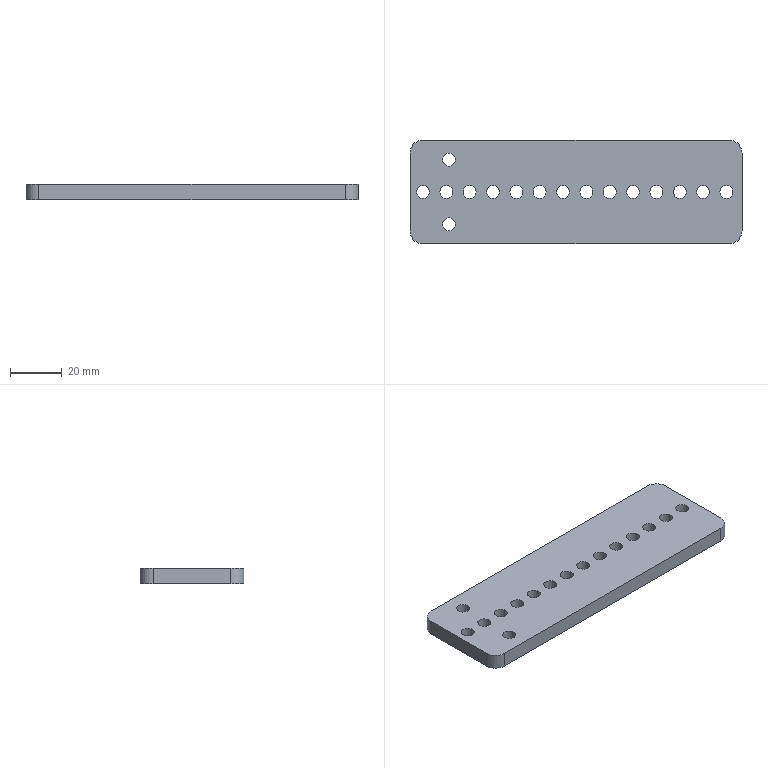Part | NX | 1 solid | 26 faces | box 128 x 40 x 6 mm | volume 28706 mm3 | cylinder 20 | plane 6 | commonest cylinder face diameters 5 x16 10 x4
STEP:
#1=CARTESIAN_POINT('',(-64.,15.,0.));
#2=VERTEX_POINT('',#1);
#3=CARTESIAN_POINT('',(-64.,-15.,0.));
#4=VERTEX_POINT('',#3);
#5=CARTESIAN_POINT('',(-64.,20.,0.));
#6=DIRECTION('',(0.,-1.,0.));
#7=VECTOR('',#6,1000.);
#8=LINE('',#5,#7);
#9=EDGE_CURVE('',#2,#4,#8,.T.);
#10=ORIENTED_EDGE('',*,*,#9,.T.);
#11=CARTESIAN_POINT('',(-64.,-15.,6.));
#12=VERTEX_POINT('',#11);
#13=CARTESIAN_POINT('',(-64.,-15.,6.));
#14=DIRECTION('',(0.,0.,-1.));
#15=VECTOR('',#14,1000.);
#16=LINE('',#13,#15);
#17=EDGE_CURVE('',#4,#12,#16,.F.);
#18=ORIENTED_EDGE('',*,*,#17,.T.);
#19=CARTESIAN_POINT('',(-64.,15.,6.));
#20=VERTEX_POINT('',#19);
#21=CARTESIAN_POINT('',(-64.,20.,6.));
#22=DIRECTION('',(0.,-1.,0.));
#23=VECTOR('',#22,1000.);
#24=LINE('',#21,#23);
#25=EDGE_CURVE('',#20,#12,#24,.T.);
#26=ORIENTED_EDGE('',*,*,#25,.F.);
#27=CARTESIAN_POINT('',(-64.,15.,6.));
#28=DIRECTION('',(0.,0.,-1.));
#29=VECTOR('',#28,1000.);
#30=LINE('',#27,#29);
#31=EDGE_CURVE('',#20,#2,#30,.T.);
#32=ORIENTED_EDGE('',*,*,#31,.T.);
#33=EDGE_LOOP('',(#10,#18,#26,#32));
#34=FACE_BOUND('',#33,.T.);
#35=CARTESIAN_POINT('',(-64.,20.,6.));
#36=DIRECTION('',(1.,0.,0.));
#37=DIRECTION('',(0.,0.,-1.));
#38=AXIS2_PLACEMENT_3D('',#35,#36,#37);
#39=PLANE('',#38);
#40=ADVANCED_FACE('',(#34),#39,.F.);
#41=CARTESIAN_POINT('',(-59.,-20.,6.));
#42=VERTEX_POINT('',#41);
#43=CARTESIAN_POINT('',(59.,-20.,6.));
#44=VERTEX_POINT('',#43);
#45=CARTESIAN_POINT('',(-64.,-20.,6.));
#46=DIRECTION('',(1.,0.,0.));
#47=VECTOR('',#46,1000.);
#48=LINE('',#45,#47);
#49=EDGE_CURVE('',#42,#44,#48,.T.);
#50=ORIENTED_EDGE('',*,*,#49,.F.);
#51=CARTESIAN_POINT('',(-59.,-20.,0.));
#52=VERTEX_POINT('',#51);
#53=CARTESIAN_POINT('',(-59.,-20.,6.));
#54=DIRECTION('',(0.,0.,-1.));
#55=VECTOR('',#54,1000.);
#56=LINE('',#53,#55);
#57=EDGE_CURVE('',#42,#52,#56,.T.);
#58=ORIENTED_EDGE('',*,*,#57,.T.);
#59=CARTESIAN_POINT('',(59.,-20.,0.));
#60=VERTEX_POINT('',#59);
#61=CARTESIAN_POINT('',(-64.,-20.,0.));
#62=DIRECTION('',(1.,0.,0.));
#63=VECTOR('',#62,1000.);
#64=LINE('',#61,#63);
#65=EDGE_CURVE('',#52,#60,#64,.T.);
#66=ORIENTED_EDGE('',*,*,#65,.T.);
#67=CARTESIAN_POINT('',(59.,-20.,6.));
#68=DIRECTION('',(0.,0.,-1.));
#69=VECTOR('',#68,1000.);
#70=LINE('',#67,#69);
#71=EDGE_CURVE('',#60,#44,#70,.F.);
#72=ORIENTED_EDGE('',*,*,#71,.T.);
#73=EDGE_LOOP('',(#50,#58,#66,#72));
#74=FACE_BOUND('',#73,.T.);
#75=CARTESIAN_POINT('',(-64.,-20.,6.));
#76=DIRECTION('',(0.,1.,0.));
#77=DIRECTION('',(-1.,0.,0.));
#78=AXIS2_PLACEMENT_3D('',#75,#76,#77);
#79=PLANE('',#78);
#80=ADVANCED_FACE('',(#74),#79,.F.);
#81=CARTESIAN_POINT('',(64.,-15.,6.));
#82=VERTEX_POINT('',#81);
#83=CARTESIAN_POINT('',(64.,15.,6.));
#84=VERTEX_POINT('',#83);
#85=CARTESIAN_POINT('',(64.,20.,6.));
#86=DIRECTION('',(0.,1.,0.));
#87=VECTOR('',#86,1000.);
#88=LINE('',#85,#87);
#89=EDGE_CURVE('',#82,#84,#88,.T.);
#90=ORIENTED_EDGE('',*,*,#89,.F.);
#91=CARTESIAN_POINT('',(64.,-15.,0.));
#92=VERTEX_POINT('',#91);
#93=CARTESIAN_POINT('',(64.,-15.,6.));
#94=DIRECTION('',(0.,0.,-1.));
#95=VECTOR('',#94,1000.);
#96=LINE('',#93,#95);
#97=EDGE_CURVE('',#82,#92,#96,.T.);
#98=ORIENTED_EDGE('',*,*,#97,.T.);
#99=CARTESIAN_POINT('',(64.,15.,0.));
#100=VERTEX_POINT('',#99);
#101=CARTESIAN_POINT('',(64.,20.,0.));
#102=DIRECTION('',(0.,1.,0.));
#103=VECTOR('',#102,1000.);
#104=LINE('',#101,#103);
#105=EDGE_CURVE('',#92,#100,#104,.T.);
#106=ORIENTED_EDGE('',*,*,#105,.T.);
#107=CARTESIAN_POINT('',(64.,15.,6.));
#108=DIRECTION('',(0.,0.,-1.));
#109=VECTOR('',#108,1000.);
#110=LINE('',#107,#109);
#111=EDGE_CURVE('',#100,#84,#110,.F.);
#112=ORIENTED_EDGE('',*,*,#111,.T.);
#113=EDGE_LOOP('',(#90,#98,#106,#112));
#114=FACE_BOUND('',#113,.T.);
#115=CARTESIAN_POINT('',(64.,20.,6.));
#116=DIRECTION('',(-1.,0.,0.));
#117=DIRECTION('',(0.,0.,1.));
#118=AXIS2_PLACEMENT_3D('',#115,#116,#117);
#119=PLANE('',#118);
#120=ADVANCED_FACE('',(#114),#119,.F.);
#121=CARTESIAN_POINT('',(59.,20.,0.));
#122=VERTEX_POINT('',#121);
#123=CARTESIAN_POINT('',(-59.,20.,0.));
#124=VERTEX_POINT('',#123);
#125=CARTESIAN_POINT('',(-64.,20.,0.));
#126=DIRECTION('',(-1.,0.,0.));
#127=VECTOR('',#126,1000.);
#128=LINE('',#125,#127);
#129=EDGE_CURVE('',#122,#124,#128,.T.);
#130=ORIENTED_EDGE('',*,*,#129,.T.);
#131=CARTESIAN_POINT('',(-59.,20.,6.));
#132=VERTEX_POINT('',#131);
#133=CARTESIAN_POINT('',(-59.,20.,6.));
#134=DIRECTION('',(0.,0.,-1.));
#135=VECTOR('',#134,1000.);
#136=LINE('',#133,#135);
#137=EDGE_CURVE('',#124,#132,#136,.F.);
#138=ORIENTED_EDGE('',*,*,#137,.T.);
#139=CARTESIAN_POINT('',(59.,20.,6.));
#140=VERTEX_POINT('',#139);
#141=CARTESIAN_POINT('',(-64.,20.,6.));
#142=DIRECTION('',(-1.,0.,0.));
#143=VECTOR('',#142,1000.);
#144=LINE('',#141,#143);
#145=EDGE_CURVE('',#140,#132,#144,.T.);
#146=ORIENTED_EDGE('',*,*,#145,.F.);
#147=CARTESIAN_POINT('',(59.,20.,6.));
#148=DIRECTION('',(0.,0.,-1.));
#149=VECTOR('',#148,1000.);
#150=LINE('',#147,#149);
#151=EDGE_CURVE('',#140,#122,#150,.T.);
#152=ORIENTED_EDGE('',*,*,#151,.T.);
#153=EDGE_LOOP('',(#130,#138,#146,#152));
#154=FACE_BOUND('',#153,.T.);
#155=CARTESIAN_POINT('',(-64.,20.,6.));
#156=DIRECTION('',(0.,-1.,0.));
#157=DIRECTION('',(1.,0.,0.));
#158=AXIS2_PLACEMENT_3D('',#155,#156,#157);
#159=PLANE('',#158);
#160=ADVANCED_FACE('',(#154),#159,.F.);
#161=CARTESIAN_POINT('',(-47.5,0.,6.));
#162=VERTEX_POINT('',#161);
#163=CARTESIAN_POINT('',(-50.,0.,6.));
#164=DIRECTION('',(0.,0.,1.));
#165=DIRECTION('',(1.,0.,0.));
#166=AXIS2_PLACEMENT_3D('',#163,#164,#165);
#167=CIRCLE('',#166,2.5);
#168=EDGE_CURVE('',#162,#162,#167,.T.);
#169=ORIENTED_EDGE('',*,*,#168,.F.);
#170=EDGE_LOOP('',(#169));
#171=FACE_BOUND('',#170,.T.);
#172=CARTESIAN_POINT('',(-56.5,0.,6.));
#173=VERTEX_POINT('',#172);
#174=CARTESIAN_POINT('',(-59.,0.,6.));
#175=DIRECTION('',(0.,0.,1.));
#176=DIRECTION('',(1.,0.,0.));
#177=AXIS2_PLACEMENT_3D('',#174,#175,#176);
#178=CIRCLE('',#177,2.5);
#179=EDGE_CURVE('',#173,#173,#178,.T.);
#180=ORIENTED_EDGE('',*,*,#179,.F.);
#181=EDGE_LOOP('',(#180));
#182=FACE_BOUND('',#181,.T.);
#183=CARTESIAN_POINT('',(-46.5,-12.5,6.));
#184=VERTEX_POINT('',#183);
#185=CARTESIAN_POINT('',(-49.,-12.5,6.));
#186=DIRECTION('',(0.,0.,1.));
#187=DIRECTION('',(1.,0.,0.));
#188=AXIS2_PLACEMENT_3D('',#185,#186,#187);
#189=CIRCLE('',#188,2.5);
#190=EDGE_CURVE('',#184,#184,#189,.T.);
#191=ORIENTED_EDGE('',*,*,#190,.F.);
#192=EDGE_LOOP('',(#191));
#193=FACE_BOUND('',#192,.T.);
#194=CARTESIAN_POINT('',(-46.5,12.5,6.));
#195=VERTEX_POINT('',#194);
#196=CARTESIAN_POINT('',(-49.,12.5,6.));
#197=DIRECTION('',(0.,0.,1.));
#198=DIRECTION('',(1.,0.,0.));
#199=AXIS2_PLACEMENT_3D('',#196,#197,#198);
#200=CIRCLE('',#199,2.5);
#201=EDGE_CURVE('',#195,#195,#200,.T.);
#202=ORIENTED_EDGE('',*,*,#201,.F.);
#203=EDGE_LOOP('',(#202));
#204=FACE_BOUND('',#203,.T.);
#205=CARTESIAN_POINT('',(-29.5,0.,6.));
#206=VERTEX_POINT('',#205);
#207=CARTESIAN_POINT('',(-32.,0.,6.));
#208=DIRECTION('',(0.,0.,1.));
#209=DIRECTION('',(1.,0.,0.));
#210=AXIS2_PLACEMENT_3D('',#207,#208,#209);
#211=CIRCLE('',#210,2.5);
#212=EDGE_CURVE('',#206,#206,#211,.T.);
#213=ORIENTED_EDGE('',*,*,#212,.F.);
#214=EDGE_LOOP('',(#213));
#215=FACE_BOUND('',#214,.T.);
#216=CARTESIAN_POINT('',(-38.5,0.,6.));
#217=VERTEX_POINT('',#216);
#218=CARTESIAN_POINT('',(-41.,0.,6.));
#219=DIRECTION('',(0.,0.,1.));
#220=DIRECTION('',(1.,0.,0.));
#221=AXIS2_PLACEMENT_3D('',#218,#219,#220);
#222=CIRCLE('',#221,2.5);
#223=EDGE_CURVE('',#217,#217,#222,.T.);
#224=ORIENTED_EDGE('',*,*,#223,.F.);
#225=EDGE_LOOP('',(#224));
#226=FACE_BOUND('',#225,.T.);
#227=ORIENTED_EDGE('',*,*,#25,.T.);
#228=CARTESIAN_POINT('',(-59.,-15.,6.));
#229=DIRECTION('',(0.,0.,1.));
#230=DIRECTION('',(1.,0.,0.));
#231=AXIS2_PLACEMENT_3D('',#228,#229,#230);
#232=CIRCLE('',#231,5.);
#233=EDGE_CURVE('',#12,#42,#232,.T.);
#234=ORIENTED_EDGE('',*,*,#233,.T.);
#235=ORIENTED_EDGE('',*,*,#49,.T.);
#236=CARTESIAN_POINT('',(59.,-15.,6.));
#237=DIRECTION('',(0.,0.,1.));
#238=DIRECTION('',(1.,0.,0.));
#239=AXIS2_PLACEMENT_3D('',#236,#237,#238);
#240=CIRCLE('',#239,5.);
#241=EDGE_CURVE('',#44,#82,#240,.T.);
#242=ORIENTED_EDGE('',*,*,#241,.T.);
#243=ORIENTED_EDGE('',*,*,#89,.T.);
#244=CARTESIAN_POINT('',(59.,15.,6.));
#245=DIRECTION('',(0.,0.,1.));
#246=DIRECTION('',(1.,0.,0.));
#247=AXIS2_PLACEMENT_3D('',#244,#245,#246);
#248=CIRCLE('',#247,5.);
#249=EDGE_CURVE('',#84,#140,#248,.T.);
#250=ORIENTED_EDGE('',*,*,#249,.T.);
#251=ORIENTED_EDGE('',*,*,#145,.T.);
#252=CARTESIAN_POINT('',(-59.,15.,6.));
#253=DIRECTION('',(0.,0.,1.));
#254=DIRECTION('',(1.,0.,0.));
#255=AXIS2_PLACEMENT_3D('',#252,#253,#254);
#256=CIRCLE('',#255,5.);
#257=EDGE_CURVE('',#132,#20,#256,.T.);
#258=ORIENTED_EDGE('',*,*,#257,.T.);
#259=EDGE_LOOP('',(#227,#234,#235,#242,#243,#250,#251,#258));
#260=FACE_BOUND('',#259,.T.);
#261=CARTESIAN_POINT('',(-20.5,0.,6.));
#262=VERTEX_POINT('',#261);
#263=CARTESIAN_POINT('',(-23.,0.,6.));
#264=DIRECTION('',(0.,0.,1.));
#265=DIRECTION('',(1.,0.,0.));
#266=AXIS2_PLACEMENT_3D('',#263,#264,#265);
#267=CIRCLE('',#266,2.5);
#268=EDGE_CURVE('',#262,#262,#267,.T.);
#269=ORIENTED_EDGE('',*,*,#268,.F.);
#270=EDGE_LOOP('',(#269));
#271=FACE_BOUND('',#270,.T.);
#272=CARTESIAN_POINT('',(-11.5,0.,6.));
#273=VERTEX_POINT('',#272);
#274=CARTESIAN_POINT('',(-14.,0.,6.));
#275=DIRECTION('',(0.,0.,1.));
#276=DIRECTION('',(1.,0.,0.));
#277=AXIS2_PLACEMENT_3D('',#274,#275,#276);
#278=CIRCLE('',#277,2.5);
#279=EDGE_CURVE('',#273,#273,#278,.T.);
#280=ORIENTED_EDGE('',*,*,#279,.F.);
#281=EDGE_LOOP('',(#280));
#282=FACE_BOUND('',#281,.T.);
#283=CARTESIAN_POINT('',(-2.5,0.,6.));
#284=VERTEX_POINT('',#283);
#285=CARTESIAN_POINT('',(-5.,0.,6.));
#286=DIRECTION('',(0.,0.,1.));
#287=DIRECTION('',(1.,0.,0.));
#288=AXIS2_PLACEMENT_3D('',#285,#286,#287);
#289=CIRCLE('',#288,2.5);
#290=EDGE_CURVE('',#284,#284,#289,.T.);
#291=ORIENTED_EDGE('',*,*,#290,.F.);
#292=EDGE_LOOP('',(#291));
#293=FACE_BOUND('',#292,.T.);
#294=CARTESIAN_POINT('',(6.5,0.,6.));
#295=VERTEX_POINT('',#294);
#296=CARTESIAN_POINT('',(4.,0.,6.));
#297=DIRECTION('',(0.,0.,1.));
#298=DIRECTION('',(1.,0.,0.));
#299=AXIS2_PLACEMENT_3D('',#296,#297,#298);
#300=CIRCLE('',#299,2.5);
#301=EDGE_CURVE('',#295,#295,#300,.T.);
#302=ORIENTED_EDGE('',*,*,#301,.F.);
#303=EDGE_LOOP('',(#302));
#304=FACE_BOUND('',#303,.T.);
#305=CARTESIAN_POINT('',(15.5,0.,6.));
#306=VERTEX_POINT('',#305);
#307=CARTESIAN_POINT('',(13.,0.,6.));
#308=DIRECTION('',(0.,0.,1.));
#309=DIRECTION('',(1.,0.,0.));
#310=AXIS2_PLACEMENT_3D('',#307,#308,#309);
#311=CIRCLE('',#310,2.5);
#312=EDGE_CURVE('',#306,#306,#311,.T.);
#313=ORIENTED_EDGE('',*,*,#312,.F.);
#314=EDGE_LOOP('',(#313));
#315=FACE_BOUND('',#314,.T.);
#316=CARTESIAN_POINT('',(24.5,0.,6.));
#317=VERTEX_POINT('',#316);
#318=CARTESIAN_POINT('',(22.,0.,6.));
#319=DIRECTION('',(0.,0.,1.));
#320=DIRECTION('',(1.,0.,0.));
#321=AXIS2_PLACEMENT_3D('',#318,#319,#320);
#322=CIRCLE('',#321,2.5);
#323=EDGE_CURVE('',#317,#317,#322,.T.);
#324=ORIENTED_EDGE('',*,*,#323,.F.);
#325=EDGE_LOOP('',(#324));
#326=FACE_BOUND('',#325,.T.);
#327=CARTESIAN_POINT('',(33.5,0.,6.));
#328=VERTEX_POINT('',#327);
#329=CARTESIAN_POINT('',(31.,0.,6.));
#330=DIRECTION('',(0.,0.,1.));
#331=DIRECTION('',(1.,0.,0.));
#332=AXIS2_PLACEMENT_3D('',#329,#330,#331);
#333=CIRCLE('',#332,2.5);
#334=EDGE_CURVE('',#328,#328,#333,.T.);
#335=ORIENTED_EDGE('',*,*,#334,.F.);
#336=EDGE_LOOP('',(#335));
#337=FACE_BOUND('',#336,.T.);
#338=CARTESIAN_POINT('',(42.5,0.,6.));
#339=VERTEX_POINT('',#338);
#340=CARTESIAN_POINT('',(40.,0.,6.));
#341=DIRECTION('',(0.,0.,1.));
#342=DIRECTION('',(1.,0.,0.));
#343=AXIS2_PLACEMENT_3D('',#340,#341,#342);
#344=CIRCLE('',#343,2.5);
#345=EDGE_CURVE('',#339,#339,#344,.T.);
#346=ORIENTED_EDGE('',*,*,#345,.F.);
#347=EDGE_LOOP('',(#346));
#348=FACE_BOUND('',#347,.T.);
#349=CARTESIAN_POINT('',(51.5,0.,6.));
#350=VERTEX_POINT('',#349);
#351=CARTESIAN_POINT('',(49.,0.,6.));
#352=DIRECTION('',(0.,0.,1.));
#353=DIRECTION('',(1.,0.,0.));
#354=AXIS2_PLACEMENT_3D('',#351,#352,#353);
#355=CIRCLE('',#354,2.5);
#356=EDGE_CURVE('',#350,#350,#355,.T.);
#357=ORIENTED_EDGE('',*,*,#356,.F.);
#358=EDGE_LOOP('',(#357));
#359=FACE_BOUND('',#358,.T.);
#360=CARTESIAN_POINT('',(60.5,0.,6.));
#361=VERTEX_POINT('',#360);
#362=CARTESIAN_POINT('',(58.,0.,6.));
#363=DIRECTION('',(0.,0.,1.));
#364=DIRECTION('',(1.,0.,0.));
#365=AXIS2_PLACEMENT_3D('',#362,#363,#364);
#366=CIRCLE('',#365,2.5);
#367=EDGE_CURVE('',#361,#361,#366,.T.);
#368=ORIENTED_EDGE('',*,*,#367,.F.);
#369=EDGE_LOOP('',(#368));
#370=FACE_BOUND('',#369,.T.);
#371=CARTESIAN_POINT('',(0.,0.,6.));
#372=DIRECTION('',(0.,0.,1.));
#373=DIRECTION('',(1.,0.,0.));
#374=AXIS2_PLACEMENT_3D('',#371,#372,#373);
#375=PLANE('',#374);
#376=ADVANCED_FACE('',(#171,#182,#193,#204,#215,#226,#260,#271,#282,#293,#304,#315,#326,#337,#348,#359,#370),#375,.T.);
#377=CARTESIAN_POINT('',(-47.5,0.,0.));
#378=VERTEX_POINT('',#377);
#379=CARTESIAN_POINT('',(-50.,0.,0.));
#380=DIRECTION('',(0.,0.,1.));
#381=DIRECTION('',(1.,0.,0.));
#382=AXIS2_PLACEMENT_3D('',#379,#380,#381);
#383=CIRCLE('',#382,2.5);
#384=EDGE_CURVE('',#378,#378,#383,.T.);
#385=ORIENTED_EDGE('',*,*,#384,.T.);
#386=EDGE_LOOP('',(#385));
#387=FACE_BOUND('',#386,.T.);
#388=CARTESIAN_POINT('',(-56.5,0.,0.));
#389=VERTEX_POINT('',#388);
#390=CARTESIAN_POINT('',(-59.,0.,0.));
#391=DIRECTION('',(0.,0.,1.));
#392=DIRECTION('',(1.,0.,0.));
#393=AXIS2_PLACEMENT_3D('',#390,#391,#392);
#394=CIRCLE('',#393,2.5);
#395=EDGE_CURVE('',#389,#389,#394,.T.);
#396=ORIENTED_EDGE('',*,*,#395,.T.);
#397=EDGE_LOOP('',(#396));
#398=FACE_BOUND('',#397,.T.);
#399=CARTESIAN_POINT('',(-46.5,-12.5,0.));
#400=VERTEX_POINT('',#399);
#401=CARTESIAN_POINT('',(-49.,-12.5,0.));
#402=DIRECTION('',(0.,0.,1.));
#403=DIRECTION('',(1.,0.,0.));
#404=AXIS2_PLACEMENT_3D('',#401,#402,#403);
#405=CIRCLE('',#404,2.5);
#406=EDGE_CURVE('',#400,#400,#405,.T.);
#407=ORIENTED_EDGE('',*,*,#406,.T.);
#408=EDGE_LOOP('',(#407));
#409=FACE_BOUND('',#408,.T.);
#410=CARTESIAN_POINT('',(-46.5,12.5,0.));
#411=VERTEX_POINT('',#410);
#412=CARTESIAN_POINT('',(-49.,12.5,0.));
#413=DIRECTION('',(0.,0.,1.));
#414=DIRECTION('',(1.,0.,0.));
#415=AXIS2_PLACEMENT_3D('',#412,#413,#414);
#416=CIRCLE('',#415,2.5);
#417=EDGE_CURVE('',#411,#411,#416,.T.);
#418=ORIENTED_EDGE('',*,*,#417,.T.);
#419=EDGE_LOOP('',(#418));
#420=FACE_BOUND('',#419,.T.);
#421=CARTESIAN_POINT('',(-29.5,0.,0.));
#422=VERTEX_POINT('',#421);
#423=CARTESIAN_POINT('',(-32.,0.,0.));
#424=DIRECTION('',(0.,0.,1.));
#425=DIRECTION('',(1.,0.,0.));
#426=AXIS2_PLACEMENT_3D('',#423,#424,#425);
#427=CIRCLE('',#426,2.5);
#428=EDGE_CURVE('',#422,#422,#427,.T.);
#429=ORIENTED_EDGE('',*,*,#428,.T.);
#430=EDGE_LOOP('',(#429));
#431=FACE_BOUND('',#430,.T.);
#432=CARTESIAN_POINT('',(-38.5,0.,0.));
#433=VERTEX_POINT('',#432);
#434=CARTESIAN_POINT('',(-41.,0.,0.));
#435=DIRECTION('',(0.,0.,1.));
#436=DIRECTION('',(1.,0.,0.));
#437=AXIS2_PLACEMENT_3D('',#434,#435,#436);
#438=CIRCLE('',#437,2.5);
#439=EDGE_CURVE('',#433,#433,#438,.T.);
#440=ORIENTED_EDGE('',*,*,#439,.T.);
#441=EDGE_LOOP('',(#440));
#442=FACE_BOUND('',#441,.T.);
#443=ORIENTED_EDGE('',*,*,#65,.F.);
#444=CARTESIAN_POINT('',(-59.,-15.,0.));
#445=DIRECTION('',(0.,0.,1.));
#446=DIRECTION('',(1.,0.,0.));
#447=AXIS2_PLACEMENT_3D('',#444,#445,#446);
#448=CIRCLE('',#447,5.);
#449=EDGE_CURVE('',#52,#4,#448,.F.);
#450=ORIENTED_EDGE('',*,*,#449,.T.);
#451=ORIENTED_EDGE('',*,*,#9,.F.);
#452=CARTESIAN_POINT('',(-59.,15.,0.));
#453=DIRECTION('',(0.,0.,1.));
#454=DIRECTION('',(1.,0.,0.));
#455=AXIS2_PLACEMENT_3D('',#452,#453,#454);
#456=CIRCLE('',#455,5.);
#457=EDGE_CURVE('',#2,#124,#456,.F.);
#458=ORIENTED_EDGE('',*,*,#457,.T.);
#459=ORIENTED_EDGE('',*,*,#129,.F.);
#460=CARTESIAN_POINT('',(59.,15.,0.));
#461=DIRECTION('',(0.,0.,1.));
#462=DIRECTION('',(1.,0.,0.));
#463=AXIS2_PLACEMENT_3D('',#460,#461,#462);
#464=CIRCLE('',#463,5.);
#465=EDGE_CURVE('',#122,#100,#464,.F.);
#466=ORIENTED_EDGE('',*,*,#465,.T.);
#467=ORIENTED_EDGE('',*,*,#105,.F.);
#468=CARTESIAN_POINT('',(59.,-15.,0.));
#469=DIRECTION('',(0.,0.,1.));
#470=DIRECTION('',(1.,0.,0.));
#471=AXIS2_PLACEMENT_3D('',#468,#469,#470);
#472=CIRCLE('',#471,5.);
#473=EDGE_CURVE('',#92,#60,#472,.F.);
#474=ORIENTED_EDGE('',*,*,#473,.T.);
#475=EDGE_LOOP('',(#443,#450,#451,#458,#459,#466,#467,#474));
#476=FACE_BOUND('',#475,.T.);
#477=CARTESIAN_POINT('',(-20.5,0.,0.));
#478=VERTEX_POINT('',#477);
#479=CARTESIAN_POINT('',(-23.,0.,0.));
#480=DIRECTION('',(0.,0.,1.));
#481=DIRECTION('',(1.,0.,0.));
#482=AXIS2_PLACEMENT_3D('',#479,#480,#481);
#483=CIRCLE('',#482,2.5);
#484=EDGE_CURVE('',#478,#478,#483,.T.);
#485=ORIENTED_EDGE('',*,*,#484,.T.);
#486=EDGE_LOOP('',(#485));
#487=FACE_BOUND('',#486,.T.);
#488=CARTESIAN_POINT('',(-11.5,0.,0.));
#489=VERTEX_POINT('',#488);
#490=CARTESIAN_POINT('',(-14.,0.,0.));
#491=DIRECTION('',(0.,0.,1.));
#492=DIRECTION('',(1.,0.,0.));
#493=AXIS2_PLACEMENT_3D('',#490,#491,#492);
#494=CIRCLE('',#493,2.5);
#495=EDGE_CURVE('',#489,#489,#494,.T.);
#496=ORIENTED_EDGE('',*,*,#495,.T.);
#497=EDGE_LOOP('',(#496));
#498=FACE_BOUND('',#497,.T.);
#499=CARTESIAN_POINT('',(-2.5,0.,0.));
#500=VERTEX_POINT('',#499);
#501=CARTESIAN_POINT('',(-5.,0.,0.));
#502=DIRECTION('',(0.,0.,1.));
#503=DIRECTION('',(1.,0.,0.));
#504=AXIS2_PLACEMENT_3D('',#501,#502,#503);
#505=CIRCLE('',#504,2.5);
#506=EDGE_CURVE('',#500,#500,#505,.T.);
#507=ORIENTED_EDGE('',*,*,#506,.T.);
#508=EDGE_LOOP('',(#507));
#509=FACE_BOUND('',#508,.T.);
#510=CARTESIAN_POINT('',(6.5,0.,0.));
#511=VERTEX_POINT('',#510);
#512=CARTESIAN_POINT('',(4.,0.,0.));
#513=DIRECTION('',(0.,0.,1.));
#514=DIRECTION('',(1.,0.,0.));
#515=AXIS2_PLACEMENT_3D('',#512,#513,#514);
#516=CIRCLE('',#515,2.5);
#517=EDGE_CURVE('',#511,#511,#516,.T.);
#518=ORIENTED_EDGE('',*,*,#517,.T.);
#519=EDGE_LOOP('',(#518));
#520=FACE_BOUND('',#519,.T.);
#521=CARTESIAN_POINT('',(15.5,0.,0.));
#522=VERTEX_POINT('',#521);
#523=CARTESIAN_POINT('',(13.,0.,0.));
#524=DIRECTION('',(0.,0.,1.));
#525=DIRECTION('',(1.,0.,0.));
#526=AXIS2_PLACEMENT_3D('',#523,#524,#525);
#527=CIRCLE('',#526,2.5);
#528=EDGE_CURVE('',#522,#522,#527,.T.);
#529=ORIENTED_EDGE('',*,*,#528,.T.);
#530=EDGE_LOOP('',(#529));
#531=FACE_BOUND('',#530,.T.);
#532=CARTESIAN_POINT('',(24.5,0.,0.));
#533=VERTEX_POINT('',#532);
#534=CARTESIAN_POINT('',(22.,0.,0.));
#535=DIRECTION('',(0.,0.,1.));
#536=DIRECTION('',(1.,0.,0.));
#537=AXIS2_PLACEMENT_3D('',#534,#535,#536);
#538=CIRCLE('',#537,2.5);
#539=EDGE_CURVE('',#533,#533,#538,.T.);
#540=ORIENTED_EDGE('',*,*,#539,.T.);
#541=EDGE_LOOP('',(#540));
#542=FACE_BOUND('',#541,.T.);
#543=CARTESIAN_POINT('',(33.5,0.,0.));
#544=VERTEX_POINT('',#543);
#545=CARTESIAN_POINT('',(31.,0.,0.));
#546=DIRECTION('',(0.,0.,1.));
#547=DIRECTION('',(1.,0.,0.));
#548=AXIS2_PLACEMENT_3D('',#545,#546,#547);
#549=CIRCLE('',#548,2.5);
#550=EDGE_CURVE('',#544,#544,#549,.T.);
#551=ORIENTED_EDGE('',*,*,#550,.T.);
#552=EDGE_LOOP('',(#551));
#553=FACE_BOUND('',#552,.T.);
#554=CARTESIAN_POINT('',(42.5,0.,0.));
#555=VERTEX_POINT('',#554);
#556=CARTESIAN_POINT('',(40.,0.,0.));
#557=DIRECTION('',(0.,0.,1.));
#558=DIRECTION('',(1.,0.,0.));
#559=AXIS2_PLACEMENT_3D('',#556,#557,#558);
#560=CIRCLE('',#559,2.5);
#561=EDGE_CURVE('',#555,#555,#560,.T.);
#562=ORIENTED_EDGE('',*,*,#561,.T.);
#563=EDGE_LOOP('',(#562));
#564=FACE_BOUND('',#563,.T.);
#565=CARTESIAN_POINT('',(51.5,0.,0.));
#566=VERTEX_POINT('',#565);
#567=CARTESIAN_POINT('',(49.,0.,0.));
#568=DIRECTION('',(0.,0.,1.));
#569=DIRECTION('',(1.,0.,0.));
#570=AXIS2_PLACEMENT_3D('',#567,#568,#569);
#571=CIRCLE('',#570,2.5);
#572=EDGE_CURVE('',#566,#566,#571,.T.);
#573=ORIENTED_EDGE('',*,*,#572,.T.);
#574=EDGE_LOOP('',(#573));
#575=FACE_BOUND('',#574,.T.);
#576=CARTESIAN_POINT('',(60.5,0.,0.));
#577=VERTEX_POINT('',#576);
#578=CARTESIAN_POINT('',(58.,0.,0.));
#579=DIRECTION('',(0.,0.,1.));
#580=DIRECTION('',(1.,0.,0.));
#581=AXIS2_PLACEMENT_3D('',#578,#579,#580);
#582=CIRCLE('',#581,2.5);
#583=EDGE_CURVE('',#577,#577,#582,.T.);
#584=ORIENTED_EDGE('',*,*,#583,.T.);
#585=EDGE_LOOP('',(#584));
#586=FACE_BOUND('',#585,.T.);
#587=CARTESIAN_POINT('',(0.,0.,0.));
#588=DIRECTION('',(0.,0.,1.));
#589=DIRECTION('',(1.,0.,0.));
#590=AXIS2_PLACEMENT_3D('',#587,#588,#589);
#591=PLANE('',#590);
#592=ADVANCED_FACE('',(#387,#398,#409,#420,#431,#442,#476,#487,#498,#509,#520,#531,#542,#553,#564,#575,#586),#591,.F.);
#593=ORIENTED_EDGE('',*,*,#233,.F.);
#594=ORIENTED_EDGE('',*,*,#17,.F.);
#595=ORIENTED_EDGE('',*,*,#449,.F.);
#596=ORIENTED_EDGE('',*,*,#57,.F.);
#597=EDGE_LOOP('',(#593,#594,#595,#596));
#598=FACE_BOUND('',#597,.T.);
#599=CARTESIAN_POINT('',(-59.,-15.,6.));
#600=DIRECTION('',(0.,0.,-1.));
#601=DIRECTION('',(-1.,0.,0.));
#602=AXIS2_PLACEMENT_3D('',#599,#600,#601);
#603=CYLINDRICAL_SURFACE('',#602,5.);
#604=ADVANCED_FACE('',(#598),#603,.T.);
#605=ORIENTED_EDGE('',*,*,#257,.F.);
#606=ORIENTED_EDGE('',*,*,#137,.F.);
#607=ORIENTED_EDGE('',*,*,#457,.F.);
#608=ORIENTED_EDGE('',*,*,#31,.F.);
#609=EDGE_LOOP('',(#605,#606,#607,#608));
#610=FACE_BOUND('',#609,.T.);
#611=CARTESIAN_POINT('',(-59.,15.,6.));
#612=DIRECTION('',(0.,0.,-1.));
#613=DIRECTION('',(-1.,0.,0.));
#614=AXIS2_PLACEMENT_3D('',#611,#612,#613);
#615=CYLINDRICAL_SURFACE('',#614,5.);
#616=ADVANCED_FACE('',(#610),#615,.T.);
#617=ORIENTED_EDGE('',*,*,#241,.F.);
#618=ORIENTED_EDGE('',*,*,#71,.F.);
#619=ORIENTED_EDGE('',*,*,#473,.F.);
#620=ORIENTED_EDGE('',*,*,#97,.F.);
#621=EDGE_LOOP('',(#617,#618,#619,#620));
#622=FACE_BOUND('',#621,.T.);
#623=CARTESIAN_POINT('',(59.,-15.,6.));
#624=DIRECTION('',(0.,0.,-1.));
#625=DIRECTION('',(-1.,0.,0.));
#626=AXIS2_PLACEMENT_3D('',#623,#624,#625);
#627=CYLINDRICAL_SURFACE('',#626,5.);
#628=ADVANCED_FACE('',(#622),#627,.T.);
#629=ORIENTED_EDGE('',*,*,#249,.F.);
#630=ORIENTED_EDGE('',*,*,#111,.F.);
#631=ORIENTED_EDGE('',*,*,#465,.F.);
#632=ORIENTED_EDGE('',*,*,#151,.F.);
#633=EDGE_LOOP('',(#629,#630,#631,#632));
#634=FACE_BOUND('',#633,.T.);
#635=CARTESIAN_POINT('',(59.,15.,6.));
#636=DIRECTION('',(0.,0.,-1.));
#637=DIRECTION('',(-1.,0.,0.));
#638=AXIS2_PLACEMENT_3D('',#635,#636,#637);
#639=CYLINDRICAL_SURFACE('',#638,5.);
#640=ADVANCED_FACE('',(#634),#639,.T.);
#641=ORIENTED_EDGE('',*,*,#439,.F.);
#642=EDGE_LOOP('',(#641));
#643=FACE_BOUND('',#642,.T.);
#644=ORIENTED_EDGE('',*,*,#223,.T.);
#645=EDGE_LOOP('',(#644));
#646=FACE_BOUND('',#645,.T.);
#647=CARTESIAN_POINT('',(-41.,0.,6.));
#648=DIRECTION('',(0.,0.,1.));
#649=DIRECTION('',(1.,0.,0.));
#650=AXIS2_PLACEMENT_3D('',#647,#648,#649);
#651=CYLINDRICAL_SURFACE('',#650,2.5);
#652=ADVANCED_FACE('',(#643,#646),#651,.F.);
#653=ORIENTED_EDGE('',*,*,#428,.F.);
#654=EDGE_LOOP('',(#653));
#655=FACE_BOUND('',#654,.T.);
#656=ORIENTED_EDGE('',*,*,#212,.T.);
#657=EDGE_LOOP('',(#656));
#658=FACE_BOUND('',#657,.T.);
#659=CARTESIAN_POINT('',(-32.,0.,6.));
#660=DIRECTION('',(0.,0.,1.));
#661=DIRECTION('',(1.,0.,0.));
#662=AXIS2_PLACEMENT_3D('',#659,#660,#661);
#663=CYLINDRICAL_SURFACE('',#662,2.5);
#664=ADVANCED_FACE('',(#655,#658),#663,.F.);
#665=ORIENTED_EDGE('',*,*,#484,.F.);
#666=EDGE_LOOP('',(#665));
#667=FACE_BOUND('',#666,.T.);
#668=ORIENTED_EDGE('',*,*,#268,.T.);
#669=EDGE_LOOP('',(#668));
#670=FACE_BOUND('',#669,.T.);
#671=CARTESIAN_POINT('',(-23.,0.,6.));
#672=DIRECTION('',(0.,0.,1.));
#673=DIRECTION('',(1.,0.,0.));
#674=AXIS2_PLACEMENT_3D('',#671,#672,#673);
#675=CYLINDRICAL_SURFACE('',#674,2.5);
#676=ADVANCED_FACE('',(#667,#670),#675,.F.);
#677=ORIENTED_EDGE('',*,*,#495,.F.);
#678=EDGE_LOOP('',(#677));
#679=FACE_BOUND('',#678,.T.);
#680=ORIENTED_EDGE('',*,*,#279,.T.);
#681=EDGE_LOOP('',(#680));
#682=FACE_BOUND('',#681,.T.);
#683=CARTESIAN_POINT('',(-14.,0.,6.));
#684=DIRECTION('',(0.,0.,1.));
#685=DIRECTION('',(1.,0.,0.));
#686=AXIS2_PLACEMENT_3D('',#683,#684,#685);
#687=CYLINDRICAL_SURFACE('',#686,2.5);
#688=ADVANCED_FACE('',(#679,#682),#687,.F.);
#689=ORIENTED_EDGE('',*,*,#506,.F.);
#690=EDGE_LOOP('',(#689));
#691=FACE_BOUND('',#690,.T.);
#692=ORIENTED_EDGE('',*,*,#290,.T.);
#693=EDGE_LOOP('',(#692));
#694=FACE_BOUND('',#693,.T.);
#695=CARTESIAN_POINT('',(-5.,0.,6.));
#696=DIRECTION('',(0.,0.,1.));
#697=DIRECTION('',(1.,0.,0.));
#698=AXIS2_PLACEMENT_3D('',#695,#696,#697);
#699=CYLINDRICAL_SURFACE('',#698,2.5);
#700=ADVANCED_FACE('',(#691,#694),#699,.F.);
#701=ORIENTED_EDGE('',*,*,#517,.F.);
#702=EDGE_LOOP('',(#701));
#703=FACE_BOUND('',#702,.T.);
#704=ORIENTED_EDGE('',*,*,#301,.T.);
#705=EDGE_LOOP('',(#704));
#706=FACE_BOUND('',#705,.T.);
#707=CARTESIAN_POINT('',(4.,0.,6.));
#708=DIRECTION('',(0.,0.,1.));
#709=DIRECTION('',(1.,0.,0.));
#710=AXIS2_PLACEMENT_3D('',#707,#708,#709);
#711=CYLINDRICAL_SURFACE('',#710,2.5);
#712=ADVANCED_FACE('',(#703,#706),#711,.F.);
#713=ORIENTED_EDGE('',*,*,#528,.F.);
#714=EDGE_LOOP('',(#713));
#715=FACE_BOUND('',#714,.T.);
#716=ORIENTED_EDGE('',*,*,#312,.T.);
#717=EDGE_LOOP('',(#716));
#718=FACE_BOUND('',#717,.T.);
#719=CARTESIAN_POINT('',(13.,0.,6.));
#720=DIRECTION('',(0.,0.,1.));
#721=DIRECTION('',(1.,0.,0.));
#722=AXIS2_PLACEMENT_3D('',#719,#720,#721);
#723=CYLINDRICAL_SURFACE('',#722,2.5);
#724=ADVANCED_FACE('',(#715,#718),#723,.F.);
#725=ORIENTED_EDGE('',*,*,#539,.F.);
#726=EDGE_LOOP('',(#725));
#727=FACE_BOUND('',#726,.T.);
#728=ORIENTED_EDGE('',*,*,#323,.T.);
#729=EDGE_LOOP('',(#728));
#730=FACE_BOUND('',#729,.T.);
#731=CARTESIAN_POINT('',(22.,0.,6.));
#732=DIRECTION('',(0.,0.,1.));
#733=DIRECTION('',(1.,0.,0.));
#734=AXIS2_PLACEMENT_3D('',#731,#732,#733);
#735=CYLINDRICAL_SURFACE('',#734,2.5);
#736=ADVANCED_FACE('',(#727,#730),#735,.F.);
#737=ORIENTED_EDGE('',*,*,#550,.F.);
#738=EDGE_LOOP('',(#737));
#739=FACE_BOUND('',#738,.T.);
#740=ORIENTED_EDGE('',*,*,#334,.T.);
#741=EDGE_LOOP('',(#740));
#742=FACE_BOUND('',#741,.T.);
#743=CARTESIAN_POINT('',(31.,0.,6.));
#744=DIRECTION('',(0.,0.,1.));
#745=DIRECTION('',(1.,0.,0.));
#746=AXIS2_PLACEMENT_3D('',#743,#744,#745);
#747=CYLINDRICAL_SURFACE('',#746,2.5);
#748=ADVANCED_FACE('',(#739,#742),#747,.F.);
#749=ORIENTED_EDGE('',*,*,#561,.F.);
#750=EDGE_LOOP('',(#749));
#751=FACE_BOUND('',#750,.T.);
#752=ORIENTED_EDGE('',*,*,#345,.T.);
#753=EDGE_LOOP('',(#752));
#754=FACE_BOUND('',#753,.T.);
#755=CARTESIAN_POINT('',(40.,0.,6.));
#756=DIRECTION('',(0.,0.,1.));
#757=DIRECTION('',(1.,0.,0.));
#758=AXIS2_PLACEMENT_3D('',#755,#756,#757);
#759=CYLINDRICAL_SURFACE('',#758,2.5);
#760=ADVANCED_FACE('',(#751,#754),#759,.F.);
#761=ORIENTED_EDGE('',*,*,#572,.F.);
#762=EDGE_LOOP('',(#761));
#763=FACE_BOUND('',#762,.T.);
#764=ORIENTED_EDGE('',*,*,#356,.T.);
#765=EDGE_LOOP('',(#764));
#766=FACE_BOUND('',#765,.T.);
#767=CARTESIAN_POINT('',(49.,0.,6.));
#768=DIRECTION('',(0.,0.,1.));
#769=DIRECTION('',(1.,0.,0.));
#770=AXIS2_PLACEMENT_3D('',#767,#768,#769);
#771=CYLINDRICAL_SURFACE('',#770,2.5);
#772=ADVANCED_FACE('',(#763,#766),#771,.F.);
#773=ORIENTED_EDGE('',*,*,#583,.F.);
#774=EDGE_LOOP('',(#773));
#775=FACE_BOUND('',#774,.T.);
#776=ORIENTED_EDGE('',*,*,#367,.T.);
#777=EDGE_LOOP('',(#776));
#778=FACE_BOUND('',#777,.T.);
#779=CARTESIAN_POINT('',(58.,0.,6.));
#780=DIRECTION('',(0.,0.,1.));
#781=DIRECTION('',(1.,0.,0.));
#782=AXIS2_PLACEMENT_3D('',#779,#780,#781);
#783=CYLINDRICAL_SURFACE('',#782,2.5);
#784=ADVANCED_FACE('',(#775,#778),#783,.F.);
#785=ORIENTED_EDGE('',*,*,#417,.F.);
#786=EDGE_LOOP('',(#785));
#787=FACE_BOUND('',#786,.T.);
#788=ORIENTED_EDGE('',*,*,#201,.T.);
#789=EDGE_LOOP('',(#788));
#790=FACE_BOUND('',#789,.T.);
#791=CARTESIAN_POINT('',(-49.,12.5,6.));
#792=DIRECTION('',(0.,0.,1.));
#793=DIRECTION('',(1.,0.,0.));
#794=AXIS2_PLACEMENT_3D('',#791,#792,#793);
#795=CYLINDRICAL_SURFACE('',#794,2.5);
#796=ADVANCED_FACE('',(#787,#790),#795,.F.);
#797=ORIENTED_EDGE('',*,*,#406,.F.);
#798=EDGE_LOOP('',(#797));
#799=FACE_BOUND('',#798,.T.);
#800=ORIENTED_EDGE('',*,*,#190,.T.);
#801=EDGE_LOOP('',(#800));
#802=FACE_BOUND('',#801,.T.);
#803=CARTESIAN_POINT('',(-49.,-12.5,6.));
#804=DIRECTION('',(0.,0.,1.));
#805=DIRECTION('',(1.,0.,0.));
#806=AXIS2_PLACEMENT_3D('',#803,#804,#805);
#807=CYLINDRICAL_SURFACE('',#806,2.5);
#808=ADVANCED_FACE('',(#799,#802),#807,.F.);
#809=ORIENTED_EDGE('',*,*,#395,.F.);
#810=EDGE_LOOP('',(#809));
#811=FACE_BOUND('',#810,.T.);
#812=ORIENTED_EDGE('',*,*,#179,.T.);
#813=EDGE_LOOP('',(#812));
#814=FACE_BOUND('',#813,.T.);
#815=CARTESIAN_POINT('',(-59.,0.,6.));
#816=DIRECTION('',(0.,0.,1.));
#817=DIRECTION('',(1.,0.,0.));
#818=AXIS2_PLACEMENT_3D('',#815,#816,#817);
#819=CYLINDRICAL_SURFACE('',#818,2.5);
#820=ADVANCED_FACE('',(#811,#814),#819,.F.);
#821=ORIENTED_EDGE('',*,*,#384,.F.);
#822=EDGE_LOOP('',(#821));
#823=FACE_BOUND('',#822,.T.);
#824=ORIENTED_EDGE('',*,*,#168,.T.);
#825=EDGE_LOOP('',(#824));
#826=FACE_BOUND('',#825,.T.);
#827=CARTESIAN_POINT('',(-50.,0.,6.));
#828=DIRECTION('',(0.,0.,1.));
#829=DIRECTION('',(1.,0.,0.));
#830=AXIS2_PLACEMENT_3D('',#827,#828,#829);
#831=CYLINDRICAL_SURFACE('',#830,2.5);
#832=ADVANCED_FACE('',(#823,#826),#831,.F.);
#833=CLOSED_SHELL('',(#40,#80,#120,#160,#376,#592,#604,#616,#628,#640,#652,#664,#676,#688,#700,#712,#724,#736,#748,#760,#772,#784,#796,#808,#820,#832));
#834=MANIFOLD_SOLID_BREP('',#833);
#835=(LENGTH_UNIT()NAMED_UNIT(*)SI_UNIT(.MILLI.,.METRE.));
#836=UNCERTAINTY_MEASURE_WITH_UNIT(LENGTH_MEASURE(0.00001),#835,'','');
#837=(NAMED_UNIT(*)PLANE_ANGLE_UNIT()SI_UNIT($,.RADIAN.));
#838=(NAMED_UNIT(*)SI_UNIT($,.STERADIAN.)SOLID_ANGLE_UNIT());
#839=(GEOMETRIC_REPRESENTATION_CONTEXT(3)GLOBAL_UNCERTAINTY_ASSIGNED_CONTEXT((#836))GLOBAL_UNIT_ASSIGNED_CONTEXT((#835,#837,#838))REPRESENTATION_CONTEXT('',''));
#840=ADVANCED_BREP_SHAPE_REPRESENTATION('',(#834),#839);